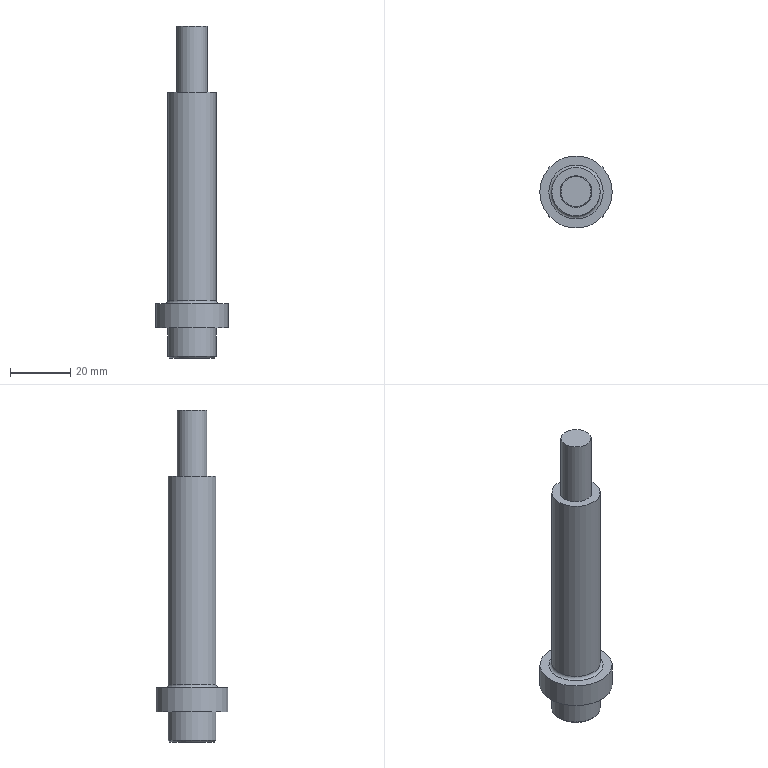Part | STEP file | 1_id222_x_t | 1 solid | 252 faces | box 24 x 24 x 110 mm | volume 20379 mm3 | plane 125 | other 119 | cylinder 5 | cone 2 | torus 1 | commonest cylinder face diameters 16 x2 10 x1 10.6 x1 24 x1